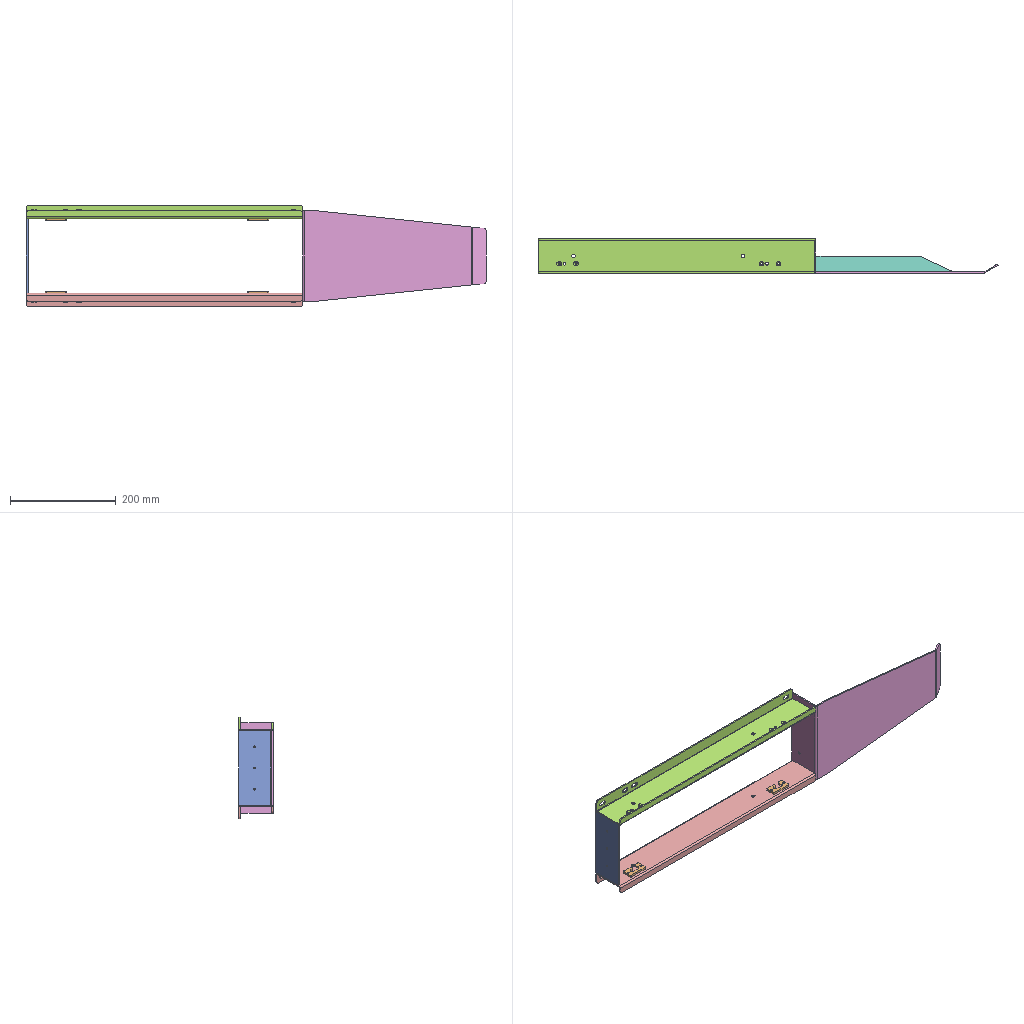Assembly | SolidWorks | 6 different items | 9 placed | box 868 x 65 x 191 mm
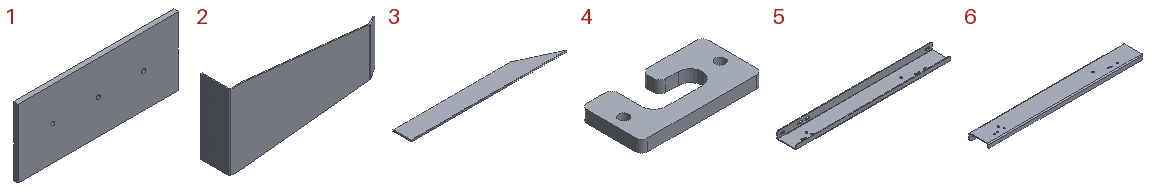Parts list (item | quantity | size | volume | features):
1 | x1 | 141 x 4 x 60 mm | 33737 mm3 | features Extrusion 1, HoleWzd 1
2 | x1 | 345.981 x 65 x 170 mm | 147766 mm3 | features Fillet 1, FlatPattern 1, HoleWzd 1, ICE 1, MirrorPattern 1, SMBaseFlange 1, SheetMetal 1
3 | x1 | 260 x 30 x 2.5 mm | 17087 mm3 | features FlatPattern 1, SMBaseFlange 1, SheetMetal 1
4 | x4 | 40 x 20 x 4 mm | 2269 mm3 | features BreakCorner 1, FlatPattern 1, HoleWzd 1, ICE 1, SMBaseFlange 1, SheetMetal 1
5 | x1 | 522 x 65 x 25 mm | 126606 mm3 | features MirrorStock 1
6 | x1 | 522 x 65 x 25 mm | 126606 mm3 | features ICE 4, BreakCorner 1, FlatPattern 1, HoleWzd 1, SMBaseFlange 1, SheetMetal 1
Mates (type | each side: item.copy, entity, surface, feature):
DistanceDim | 6.1 plane | assembly plane
Coincident | 6.1 face plane Base-Flange1 | 1.1 face plane Boss-Extrude1 | 3 times
Coincident | 6.1 face plane Base-Flange1 | 2.1 face plane Base-Flange1 | 2 times
Width | 2.1 face plane Base-Flange1 | 2.1 face plane Base-Flange1 | 6.1 face plane Base-Flange1 | 5.1 face plane 190301-01-600-01 Mirror
Coincident | 2.1 face plane Base-Flange1 | 3.1 face plane Base-Flange1 | 2 times
Width | 3.1 face plane Base-Flange1 | 3.1 face plane Base-Flange1 | 6.1 face plane Base-Flange1 | 5.1 face plane 190301-01-600-01 Mirror
Coincident | 6.1 face plane Base-Flange1 | 4.1 face plane Base-Flange1
Concentric | 6.1 face cylinder CSK for M4 Hex Socket Countersunk Cap Screw1 | 4.1 face cylinder M4 Tapped Hole1 | 2 times
Concentric | 6.1 face cylinder CSK for M4 Hex Socket Countersunk Cap Screw1 | 4.2 face cylinder M4 Tapped Hole1 | 2 times
Coincident | 6.1 face plane Base-Flange1 | 4.2 face plane Base-Flange1
Concentric | 4.1 face cylinder Cut-Extrude1 | assembly face
Concentric | 4.3 face cylinder Cut-Extrude1 | assembly face
Width | assembly face | assembly face | 5.1 face plane 190301-01-600-01 Mirror | 6.1 face plane Base-Flange1